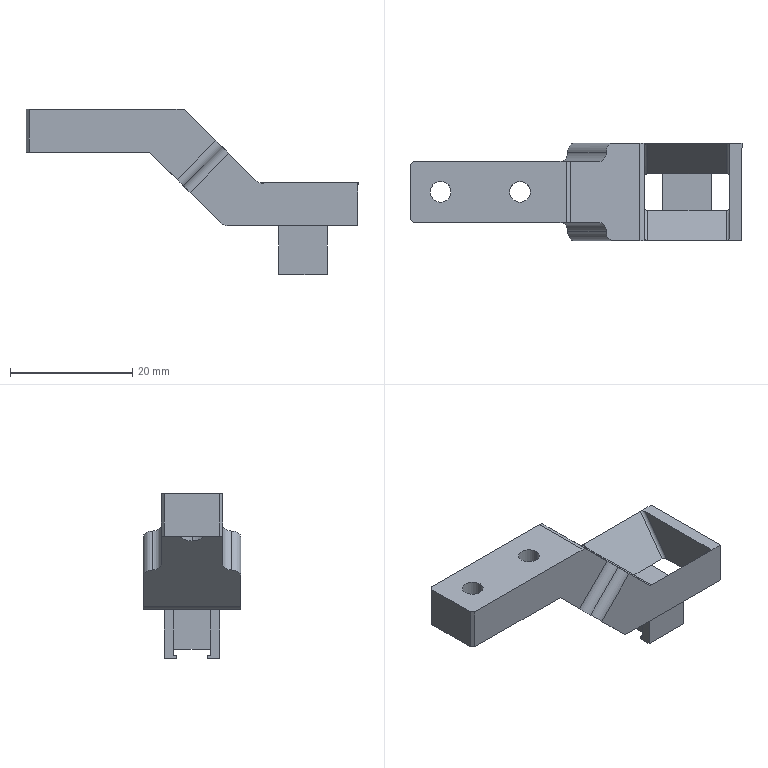NC program | NX | posted with a generic post | part box 54.3 x 16 x 27 mm
Lines 1 to 577 of 2261:
N10 G17 G21 G94 G90
(FLOOR_WALL , TOOL : D63)
N12 T01 M6
N14 G54
N16 G17 G0 G90 X-64.65 Y0. S6500 M3
N18 G43 Z30. H1
N20 Z3.
N22 G94 G1 Z0. F1250.
N24 X-61.65
N26 X61.65
N28 X64.65
N30 Z3.
N32 G0 Z30.
N34 M5
(DRILLING_COPY_1 , TOOL : D6A45)
N36 T07 M6
N38 G54
N40 G17 G0 G90 X-22.15 Y0. S5000 M3
N42 G43 Z30. H7
N44 G94 G81 G98 Z-1. F250. R3.
N46 X-9.15
N48 G80
N50 G0 X-9.15 Y0. Z30.
N52 M5
(DRILLING_COPY_COPY_1 , TOOL : 3.4ZT)
N54 T13 M6
N56 G54
N58 G17 G0 G90 X-22.15 Y0. S2000 M3
N60 G43 Z30. H13
N62 G94 G83 G98 Z-9.021 F120. Q2. R3.
N64 X-9.15
N66 G80
N68 G0 X-9.15 Y0. Z30.
N70 M5
(ZLEVEL_PROFILE_COPY_COPY_1_COPY_COPY , TOOL : D6)
N72 T06 M6
N74 G54
N76 G17 G0 G90 X-1.959 Y-8.743 S9500 M3
N78 G43 Z30. H6
N80 Z-7.182
N82 G94 G1 Z-10.182 F1200.
N84 X-1.844 Y-8.594
N86 G3 X-1.762 Y-8. R0.6
N88 G1 X-26.65
N90 X-26.914 Y-7.999
N92 X-29.773
N94 G3 X-30.292 Y-8.299 R0.6
N96 G1 X-30.393 Y-8.474
N98 Z-7.182
N100 G0 Z30.
N102 X-30.394 Y8.476
N104 Z-7.182
N106 G1 Z-10.182
N108 X-30.292 Y8.3
N110 G3 X-29.773 Y8. R0.6
N112 G1 X-24.722
N114 X-1.762
N116 G3 X-1.844 Y8.594 R0.6
N118 G1 X-1.959 Y8.743
N120 Z-7.182
N122 G0 Z30.
(FLOOR_WALL_1 , TOOL : D6)
N124 X20.308 Y-9.357
N126 Z-10.5
N128 G1 Z-12. F1250.
N130 X21.35 Y-8.755
N132 G3 X21.65 Y-8.235 R0.6
N134 G1 Y8.235
N136 X22.083 Y11.
N138 X23.2
N140 Y-11.
N142 X24.75
N144 Y11.
N146 G3 X24.45 Y11.52 R0.6
N148 G1 X22.752 Y12.5
N150 Z-10.5
N152 G0 Z30.
(FIXED_CONTOUR , TOOL : D6)
N154 X18.524 Y5.506
N156 Z-8.4
N158 G1 Z-11.544 F500.
N160 G3 X19.041 Y5.203 R0.6
N162 G1 X21.804 Y5.185 Z-11.569 F2500.
N164 X22.029 Y5.189 Z-11.563
N166 X22.05 Y5.183 Z-11.534
N168 X22.051 Y5.001 Z-11.529
N170 X22.05 Y-4.466 Z-11.617
N172 Y-5.107 Z-11.646
N174 X22.018 Y-5.14 Z-11.632
N176 X14.509 Y-5.109 Z-11.675
N178 X14.298 Y-5.106 Z-11.68
N180 X14.252 Y-5.088 Z-11.704
N182 X14.25 Y-4.438 Z-11.691
N184 X14.251 Y4.623 Z-11.769
N186 Y5.015 Z-11.786
N188 X14.327 Y5.058 Z-11.746
N190 X21.881 Y5.011 Z-11.812
N192 X22.047 Y5.001 Z-11.825
N194 X22.05 Y-4.491 Z-11.916
N196 X22.051 Y-4.716 Z-11.923
N198 X22.038 Y-4.927 Z-11.93
N200 X21.93 Y-4.967 Z-11.874
N202 X14.425 Y-4.936 Z-11.918
N204 X14.25 Y-4.875 Z-11.993
N206 Y-4.257 Z-11.988
N208 X14.251 Y4.63 Z-12.065
N210 X14.264 Y4.828 Z-12.069
N212 X14.416 Y4.885 Z-11.988
N214 X21.912 Y4.838 Z-12.054
N216 X22.05 Y4.772 Z-12.122
N218 X22.051 Y-4.59 Z-12.215
N220 X22.05 Y-4.716 Z-12.221
N222 X21.873 Y-4.783 Z-12.131
N224 X21.771 Y-4.794 Z-12.116
N226 X14.479 Y-4.763 Z-12.16
N228 X14.293 Y-4.69 Z-12.262
N230 X14.25 Y-4.655 Z-12.283
N232 X14.251 Y4.466 Z-12.36
N234 X14.263 Y4.622 Z-12.358
N236 X14.443 Y4.69 Z-12.262
N238 X14.534 Y4.712 Z-12.231
N240 X21.637 Y4.666 Z-12.294
N242 X21.857 Y4.657 Z-12.307
N244 X22.044 Y4.577 Z-12.42
N246 X22.05 Y4.163 Z-12.426
N248 X22.051 Y-4.388 Z-12.509
N250 X22.042 Y-4.514 Z-12.508
N252 X21.863 Y-4.582 Z-12.412
N254 X21.722 Y-4.621 Z-12.358
N256 X14.713 Y-4.591 Z-12.401
N258 X14.554 Y-4.585 Z-12.41
N260 X14.385 Y-4.519 Z-12.502
N262 X14.25 Y-4.453 Z-12.578
N264 X14.251 Y4.406 Z-12.657
N266 X14.43 Y4.479 Z-12.557
N268 X14.619 Y4.539 Z-12.473
N270 X21.718 Y4.493 Z-12.538
N272 X21.904 Y4.423 Z-12.634
N274 X22.05 Y4.346 Z-12.719
N276 Y-4.25 Z-12.806
N278 X22.028 Y-4.308 Z-12.797
N280 X21.85 Y-4.381 Z-12.694
N282 X21.67 Y-4.448 Z-12.6
N284 X14.701 Y-4.417 Z-12.644
N286 X14.61 Y-4.399 Z-12.669
N288 X14.272 Y-4.259 Z-12.865
N290 X14.25 Y-4.193 Z-12.878
N292 X14.251 Y4.065 Z-12.953
N294 X14.256 Y4.197 Z-12.952
N296 X14.602 Y4.337 Z-12.756
N298 X14.717 Y4.366 Z-12.715
N300 X21.536 Y4.321 Z-12.778
N302 X21.665 Y4.312 Z-12.791
N304 X22.009 Y4.166 Z-12.995
N306 X22.05 Y4.129 Z-13.018
N308 X22.051 Y-3.939 Z-13.102
N310 X22.04 Y-4.092 Z-13.099
N312 X21.583 Y-4.275 Z-12.843
N314 X14.957 Y-4.245 Z-12.885
N316 X14.733 Y-4.24 Z-12.893
N318 X14.283 Y-4.051 Z-13.157
N320 X14.25 Y-4.013 Z-13.175
N322 X14.251 Y3.819 Z-13.249
N324 X14.258 Y3.986 Z-13.248
N326 X14.611 Y4.131 Z-13.045
N328 X14.792 Y4.193 Z-12.957
N330 X21.468 Y4.148 Z-13.02
N332 X21.573 Y4.138 Z-13.035
N334 X21.918 Y3.991 Z-13.239
N336 X22.05 Y3.918 Z-13.316
N338 Y-3.837 Z-13.399
N340 X22.033 Y-3.883 Z-13.391
N342 X21.5 Y-4.1 Z-13.087
N344 X20.821 Z-13.088
N346 X14.928 Y-4.072 Z-13.128
N348 X14.812 Y-4.062 Z-13.141
N350 X14.312 Y-3.851 Z-13.437
N352 X14.25 Y-3.82 Z-13.473
N354 X14.251 Y3.604 Z-13.545
N356 X14.264 Y3.776 Z-13.541
N358 X14.797 Y3.995 Z-13.235
N360 X14.882 Y4.02 Z-13.199
N362 X21.265 Y3.977 Z-13.261
N364 X21.476 Y3.966 Z-13.276
N366 X22.045 Y3.723 Z-13.615
N368 X22.05 Y2.982 Z-13.624
N370 Y-3.563 Z-13.694
N372 X22.035 Y-3.671 Z-13.688
N374 X21.399 Y-3.93 Z-13.325
N376 X14.936 Y-3.898 Z-13.371
N378 X14.45 Y-3.696 Z-13.654
N380 X14.27 Y-3.619 Z-13.762
N382 X14.25 Y-3.557 Z-13.773
N384 X14.251 Y3.481 Z-13.842
N386 X14.269 Y3.568 Z-13.833
N388 X14.78 Y3.776 Z-13.541
N390 X14.971 Y3.847 Z-13.441
N392 X21.208 Y3.804 Z-13.503
N394 X21.378 Y3.794 Z-13.516
N396 X21.893 Y3.575 Z-13.822
N398 X22.05 Y3.492 Z-13.915
N400 Y-3.452 Z-13.99
N402 X21.3 Y-3.758 Z-13.567
N404 X15.069 Y-3.726 Z-13.612
N406 X14.988 Y-3.711 Z-13.633
N408 X14.25 Y-3.396 Z-14.07
N410 X14.251 Y3.237 Z-14.137
N412 X14.259 Y3.352 Z-14.135
N414 X14.917 Y3.62 Z-13.76
N416 X15.083 Y3.674 Z-13.684
N418 X21.158 Y3.631 Z-13.745
N420 X21.282 Y3.622 Z-13.757
N422 X21.957 Y3.335 Z-14.159
N424 X22.05 Y3.279 Z-14.214
N426 Y-3.176 Z-14.285
N428 X22.039 Y-3.247 Z-14.282
N430 X21.221 Y-3.58 Z-13.816
N432 X20.836 Y-3.583 Z-13.812
N434 X15.119 Y-3.553 Z-13.854
N436 X14.34 Y-3.223 Z-14.316
N438 X14.25 Y-3.179 Z-14.369
N440 X14.251 Y2.994 Z-14.433
N442 X14.262 Y3.142 Z-14.429
N444 X15.066 Y3.469 Z-13.971
N446 X15.177 Y3.501 Z-13.926
N448 X21.129 Y3.458 Z-13.987
N450 X21.204 Y3.442 Z-14.01
N452 X22.014 Y3.097 Z-14.491
N454 X22.05 Y3.061 Z-14.513
N456 Y-2.9 Z-14.581
N458 X22.036 Y-3.037 Z-14.576
N460 X21.208 Y-3.373 Z-14.105
N462 X21.103 Y-3.412 Z-14.051
N464 X15.214 Y-3.38 Z-14.096
N466 X14.29 Y-2.987 Z-14.646
N468 X14.251 Y-2.95 Z-14.668
N470 Y2.912 Z-14.729
N472 X14.419 Y2.995 Z-14.635
N474 X15.189 Y3.308 Z-14.197
N476 X15.252 Y3.329 Z-14.168
N478 X20.942 Y3.286 Z-14.227
N480 X21.083 Y3.28 Z-14.236
N482 X22.05 Y2.865 Z-14.812
N484 X22.046 Y-2.821 Z-14.878
N486 X21.105 Y-3.204 Z-14.343
N488 X20.993 Y-3.239 Z-14.293
N490 X15.486 Y-3.209 Z-14.336
N492 X15.292 Y-3.2 Z-14.347
N494 X14.288 Y-2.773 Z-14.946
N496 X14.251 Y-2.74 Z-14.967
N498 Y2.709 Z-15.026
N500 X14.666 Y2.884 Z-14.791
N502 X15.19 Y3.096 Z-14.493
N504 X15.354 Y3.156 Z-14.41
N506 X20.947 Y3.113 Z-14.47
N508 X21.122 Y3.05 Z-14.558
N510 X22.05 Y2.65 Z-15.111
N512 Y-2.603 Z-15.174
N514 X21.756 Y-2.729 Z-15.007
N516 X20.92 Y-3.066 Z-14.536
N518 X15.404 Y-3.035 Z-14.579
N520 X14.418 Y-2.616 Z-15.166
N522 X14.251 Y-2.528 Z-15.265
N524 Y2.502 Z-15.321
N526 X15.322 Y2.939 Z-14.714
N528 X15.448 Y2.983 Z-14.652
N530 X20.879 Y2.94 Z-14.712
N532 X21.892 Y2.508 Z-15.316
N534 X22.05 Y2.425 Z-15.41
N536 Y-2.312 Z-15.468
N538 X22.035 Y-2.403 Z-15.463
N540 X20.938 Y-2.849 Z-14.84
N542 X20.796 Y-2.893 Z-14.777
N544 X15.677 Y-2.863 Z-14.82
N546 X15.48 Y-2.854 Z-14.832
N548 X14.406 Y-2.397 Z-15.472
N550 X14.251 Y-2.316 Z-15.564
N552 Y2.204 Z-15.616
N554 X14.261 Y2.296 Z-15.613
N556 X15.502 Y2.8 Z-14.908
N558 X15.668 Y2.809 Z-14.896
N560 X20.784 Y2.768 Z-14.953
N562 X21.992 Y2.252 Z-15.675
N564 X22.047 Y2.226 Z-15.711
N566 X22.05 Y1.378 Z-15.719
N568 Y-2.068 Z-15.763
N570 X22.038 Y-2.191 Z-15.76
N572 X20.733 Y-2.719 Z-15.022
N574 X16.829 Y-2.697 Z-15.052
N576 X15.592 Y-2.688 Z-15.065
N578 X14.259 Y-2.118 Z-15.862
N580 X14.251 Y-1.909 Z-15.866
N582 X14.254 Y2.082 Z-15.914
N584 X15.473 Y2.577 Z-15.22
N586 X15.637 Y2.637 Z-15.137
N588 X20.554 Y2.596 Z-15.193
N590 X20.701 Y2.589 Z-15.203
N592 X21.901 Y2.078 Z-15.919
N594 X22.05 Y1.996 Z-16.009
N596 Y-1.967 Z-16.061
N598 X21.901 Y-2.037 Z-15.976
N600 X20.825 Y-2.472 Z-15.367
N602 X20.627 Y-2.548 Z-15.261
N604 X15.762 Y-2.517 Z-15.304
N606 X15.657 Y-2.503 Z-15.324
N608 X14.405 Y-1.97 Z-16.071
N610 X14.251 Y-1.897 Z-16.164
N612 Y1.86 Z-16.209
N614 X14.383 Y1.925 Z-16.133
N616 X15.598 Y2.416 Z-15.445
N618 X15.745 Y2.464 Z-15.379
N620 X20.36 Y2.425 Z-15.433
N622 X20.607 Y2.416 Z-15.445
N624 X21.977 Y1.831 Z-16.264
N626 X22.05 Y1.781 Z-16.309
N628 Y-1.703 Z-16.356
N630 X22.042 Y-1.766 Z-16.355
N632 X21.546 Y-1.97 Z-16.07
N634 X20.679 Y-2.32 Z-15.581
N636 X20.51 Y-2.375 Z-15.503
N638 X15.781 Y-2.343 Z-15.548
N640 X14.297 Y-1.708 Z-16.437
N642 X14.251 Y-1.674 Z-16.464
N644 Y1.609 Z-16.503
N646 X14.26 Y1.661
N648 X14.802 Y1.883 Z-16.192
N650 X15.775 Y2.276 Z-15.641
N652 X15.839 Y2.291 Z-15.621
N654 X20.271 Y2.253 Z-15.674
N656 X20.518 Y2.241 Z-15.691
N658 X21.93 Y1.638 Z-16.535
N660 X22.047 Y1.584 Z-16.609
N662 X22.05 Y-0.604 Z-16.637
N664 Y-1.398 Z-16.648
N666 X22.037 Y-1.557
N668 X21.749 Y-1.677 Z-16.48
N670 X20.516 Y-2.174 Z-15.784
N672 X20.405 Y-2.202 Z-15.745
N674 X16.052 Y-2.173 Z-15.786
N676 X15.857 Y-2.162 Z-15.801
N678 X14.339 Y-1.514 Z-16.708
N680 X14.251 Y-1.459 Z-16.766
N682 Y-0.852 Z-16.769
N684 Y1.374 Z-16.798
N686 X14.265 Y1.451 Z-16.797
N688 X14.556 Y1.573 Z-16.626
N690 X15.897 Y2.114 Z-15.868
N692 X16.347
N694 X20.184 Y2.08 Z-15.916
N696 X20.422 Y2.069 Z-15.932
N698 X22.001 Y1.394 Z-16.877
N700 X22.05 Y1.35 Z-16.91
N702 Y-0.523 Z-16.933
N704 Y-1.263 Z-16.946
N706 X22.034 Y-1.346 Z-16.943
N708 X21.768 Y-1.459 Z-16.786
N710 X20.525 Y-1.959 Z-16.085
N712 X20.331 Y-2.03 Z-15.987
N714 X15.971 Y-1.997 Z-16.031
N716 X14.354 Y-1.307 Z-16.998
N718 X14.256 Y-1.257 Z-17.069
N720 X14.251 Y-1.091 Z-17.062
N722 Y1.105 Z-17.092
N724 X14.265 Y1.238 Z-17.095
N726 X14.498 Y1.338 Z-16.954
N728 X15.841 Y1.88 Z-16.196
N730 X16.027 Y1.945 Z-16.105
N732 X20.072 Y1.908 Z-16.157
N734 X20.316 Y1.901 Z-16.167
N736 X22.027 Y1.168 Z-17.192
N738 X22.05 Y1.125 Z-17.213
N740 Y0.805 Z-17.211
N742 Y-1.018 Z-17.238
N744 X22.041 Y-1.129 Z-17.248
N746 X21.902 Y-1.194 Z-17.156
N748 X20.419 Y-1.791 Z-16.321
N750 X20.238 Y-1.857 Z-16.228
N752 X16.066 Y-1.825 Z-16.273
N754 X14.331 Y-1.081 Z-17.315
N756 X14.251 Y-1.025 Z-17.371
N758 Y-0.851 Z-17.362
N760 Y0.984 Z-17.388
N762 X14.276 Y1.03 Z-17.385
N764 X14.419 Y1.096 Z-17.294
N766 X15.94 Y1.709 Z-16.435
N768 X16.121 Y1.772 Z-16.347
N770 X20.068 Y1.735 Z-16.399
N772 X20.22 Y1.729 Z-16.408
N774 X21.936 Y0.993 Z-17.437
N776 X22.05 Y0.925 Z-17.52
N778 Y0.76 Z-17.508
N780 Y-0.762 Z-17.531
N782 X22.044 Y-0.912 Z-17.551
N784 X21.939 Y-0.969 Z-17.471
N786 X20.236 Y-1.654 Z-16.513
N788 X20.144 Y-1.684 Z-16.47
N790 X16.162 Y-1.653 Z-16.514
N792 X14.477 Y-0.932 Z-17.524
N794 X14.33 Y-0.865 Z-17.617
N796 X14.251 Y-0.812 Z-17.677
N798 Y-0.652 Z-17.662
N800 Y0.678 Z-17.681
N802 Y0.802 Z-17.7
N804 X14.392 Y0.875 Z-17.604
N806 X16.046 Y1.541 Z-16.671
N808 X16.21 Y1.599 Z-16.59
N810 X20.114 Y1.561 Z-16.642
N812 X22.004 Y0.75 Z-17.777
N814 X22.05 Y0.699 Z-17.823
N816 Y0.531 Z-17.808
N818 Y-0.538 Z-17.825
N820 Y-0.692 Z-17.855
N822 X21.968 Y-0.747 Z-17.782
N824 X20.126 Y-1.487 Z-16.747
N826 X20.031 Y-1.511 Z-16.712
N828 X16.257 Y-1.48 Z-16.756
N830 X14.432 Y-0.698 Z-17.85
N832 X14.292 Y-0.625 Z-17.953
N834 X14.251 Y-0.587 Z-17.978
N836 Y-0.465 Z-17.961
N838 Y0.499 Z-17.976
N840 X14.264 Y0.595 Z-17.995
N842 X14.366 Y0.654 Z-17.913
N844 X16.162 Y1.376 Z-16.901
N846 X16.304 Y1.426 Z-16.832
N848 X20.018 Y1.389 Z-16.884
N850 X21.976 Y0.548 Z-18.061
N852 X22.044 Y0.5 Z-18.129
N854 X22.05 Y0.329 Z-18.108
N856 Y-0.334 Z-18.119
N858 X22.041 Y-0.485 Z-18.149
N860 X21.984 Y-0.531 Z-18.085
N862 X19.969 Y-1.339 Z-16.954
N864 X16.525 Y-1.31 Z-16.994
N866 X16.333 Y-1.3 Z-17.009
N868 X14.461 Y-0.497 Z-18.133
N870 X14.334 Y-0.436 Z-18.218
N872 X14.251 Y-0.369 Z-18.286
N874 Y-0.311 Z-18.26
N876 Y0.321 Z-18.27
N878 X14.261 Y0.376 Z-18.301
N880 X14.387 Y0.452 Z-18.195
N882 X16.186 Y1.175 Z-17.183
N884 X16.4 Y1.253 Z-17.074
N886 X19.724 Y1.219 Z-17.122
N888 X19.942 Y1.208 Z-17.136
N890 X22.019 Y0.315 Z-18.387
N892 X22.05 Y0.256 Z-18.442
N894 Y0.127 Z-18.408
N896 Y-0.03 Z-18.411
N898 Y-0.187 Z-18.432
N900 X22.042 Y-0.268 Z-18.453
N902 X21.998 Y-0.315 Z-18.386
N904 X19.972 Y-1.127 Z-17.25
N906 X19.849 Y-1.166 Z-17.196
N908 X16.474 Y-1.136 Z-17.237
N910 X16.244 Y-1.048 Z-17.36
N912 X14.402 Y-0.257 Z-18.468
N914 X14.26 Y-0.161 Z-18.602
N916 X14.251 Y-0.112 Z-18.56
N918 Y0.066 Z-18.563
N920 Y0.133 Z-18.582
N922 X14.26 Y0.154 Z-18.61
N924 X14.384 Y0.241 Z-18.49
N926 X16.254 Y0.991 Z-17.44
N928 X16.494 Y1.08 Z-17.316
N930 X19.512 Y1.048 Z-17.361
N932 X19.846 Y1.036 Z-17.377
N934 X21.884 Y0.164 Z-18.598
N936 X22.017 Y0.104 Z-18.682
N938 X22.037 Y0.001 Z-18.812
N940 X21.975 Y-0.114 Z-18.668
N942 X19.813 Y-0.98 Z-17.457
N944 X19.755 Y-0.993 Z-17.438
N946 X16.819 Y-0.966 Z-17.475
N948 X16.533 Y-0.959 Z-17.485
N950 X14.621 Y-0.146 Z-18.624
N952 X14.352 Y-0.036 Z-18.777
N954 X14.341 Y0.009 Z-18.816
N956 X14.351 Y0.04 Z-18.772
N958 X14.461 Y0.061 Z-18.742
N960 X16.551 Y0.9 Z-17.569
N962 X16.783 Y0.905 Z-17.561
N964 X19.664 Y0.873 Z-17.606
N966 X19.743 Y0.867 Z-17.614
N968 X21.196 Y0.244 Z-18.487
N970 X21.448 Y0.142 Z-18.629
N972 X21.933 Y0.001 Z-18.826
N974 X21.417 Y-0.132 Z-18.644
N976 X19.677 Y-0.821 Z-17.678
N978 X16.94 Y-0.794 Z-17.716
N980 X16.624 Y-0.785 Z-17.729
N982 X15.212 Y-0.183 Z-18.572
N984 X14.65 Y0. Z-18.828
N986 X15.141 Y0.128 Z-18.649
N988 X16.49 Y0.666 Z-17.896
N990 X16.682 Y0.735 Z-17.798
N992 X19.635 Y0.699 Z-17.849
N994 X20.701 Y0.241 Z-18.49
N996 X20.936 Y0.144 Z-18.626
N998 X21.4 Y0. Z-18.827
N1000 X20.905 Y-0.132 Z-18.644
N1002 X19.584 Y-0.652 Z-17.916
N1004 X16.734 Y-0.618 Z-17.963
N1006 X15.654 Y-0.159 Z-18.606
N1008 X15.155 Y0. Z-18.828
N1010 X15.651 Y0.127 Z-18.649
N1012 X16.607 Y0.506 Z-18.12
N1014 X16.787 Y0.565 Z-18.036
N1016 X19.301 Y0.53 Z-18.086
N1018 X19.549 Y0.522 Z-18.097
N1020 X20.415 Y0.151 Z-18.617
N1022 X20.893 Y0.001 Z-18.827
N1024 X20.399 Y-0.131 Z-18.645
N1026 X19.498 Y-0.483 Z-18.151
N1028 X16.966 Y-0.447 Z-18.202
N1030 X16.817 Y-0.44 Z-18.212
N1032 X16.154 Y-0.161 Z-18.603
N1034 X15.665 Y0. Z-18.828
N1036 X16.154 Y0.125 Z-18.653
N1038 X16.597 Y0.298 Z-18.411
N1040 X16.878 Y0.397 Z-18.272
N1042 X19.025 Y0.361 Z-18.322
N1044 X19.464 Y0.344 Z-18.346
N1046 X19.929 Y0.145 Z-18.625
N1048 X20.387 Y0.001 Z-18.826
N1050 X19.871 Y-0.137 Z-18.636
N1052 X19.406 Y-0.317 Z-18.384
N1054 X16.917 Y-0.269 Z-18.451
N1056 X16.63 Y-0.15 Z-18.618
N1058 X16.166 Y0. Z-18.828
N1060 X16.662 Y0.124 Z-18.654
N1062 X16.97 Y0.231 Z-18.505
N1064 X19.348 Y0.18 Z-18.576
N1066 X19.522 Y0.104 Z-18.683
N1068 X19.883 Y0.001 Z-18.826
N1070 X19.481 Y-0.097 Z-18.692
N1072 X19.317 Y-0.156 Z-18.61
N1074 X17.693 Y-0.116 Z-18.665
N1076 X17.011 Y-0.095 Z-18.695
N1078 X16.922 Y-0.056 Z-18.749
N1080 X16.87 Y-0.042 Z-18.769
N1082 X16.673 Y0. Z-18.828
N1084 X16.915 Y0.032 Z-18.783
N1086 X17.056 Y0.069 Z-18.731
N1088 X19.024 Y0.015 Z-18.806
N1090 X19.289 Y0.002 Z-18.826
N1092 X19.241 Y-0.018 Z-18.803
N1094 X19.193 Y-0.019
N1096 X19.205 Y-0.066
N1098 Z-9.953
N1100 G0 Z-7.553
N1102 X19.185 Y0.062
N1104 Z-9.953
N1106 G1 Z-18.826 F500.
N1108 X19.214 Y-0.008
N1110 X19.289 Y0.002
N1112 X19.426 F2500.
N1114 X19.501 Y-0.008
N1116 X19.53 Y0.062
N1118 Z-9.6
N1120 G0 Z30.
N1122 M5